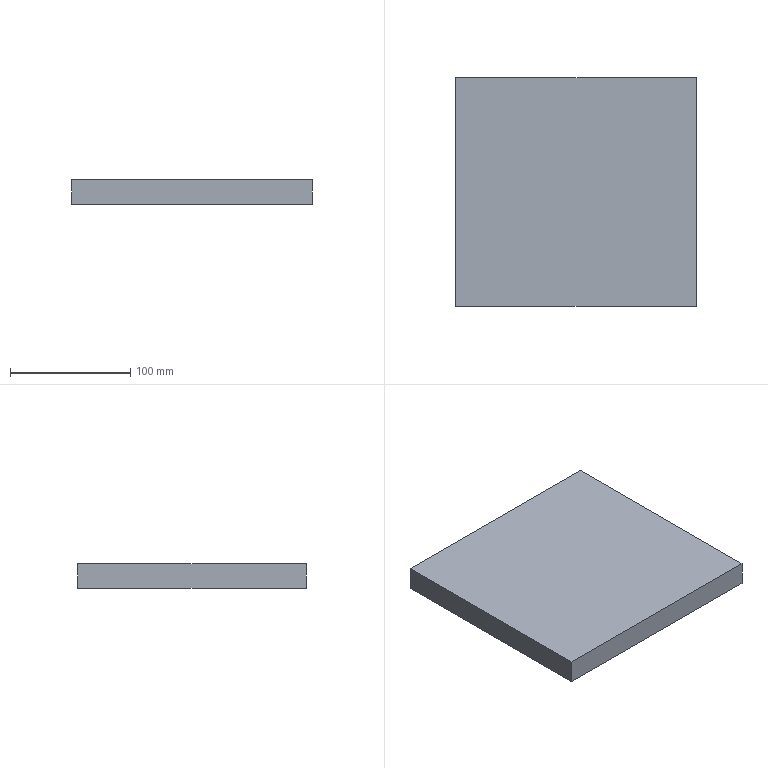Part | NX | features DATUM_CSYS 2, EXTRUDE 1, SKETCH 1 | 1 solid | 6 faces | box 200 x 190 x 20 mm | volume 760000 mm3 | plane 6
STEP:
#1=CARTESIAN_POINT('',(-100.,95.,0.));
#2=VERTEX_POINT('',#1);
#3=CARTESIAN_POINT('',(-100.,-95.,0.));
#4=VERTEX_POINT('',#3);
#5=CARTESIAN_POINT('',(-100.,95.,0.));
#6=DIRECTION('',(0.,-1.,0.));
#7=VECTOR('',#6,1000.);
#8=LINE('',#5,#7);
#9=EDGE_CURVE('',#2,#4,#8,.T.);
#10=ORIENTED_EDGE('',*,*,#9,.T.);
#11=CARTESIAN_POINT('',(-100.,-95.,20.));
#12=VERTEX_POINT('',#11);
#13=CARTESIAN_POINT('',(-100.,-95.,20.));
#14=DIRECTION('',(0.,0.,-1.));
#15=VECTOR('',#14,1000.);
#16=LINE('',#13,#15);
#17=EDGE_CURVE('',#12,#4,#16,.T.);
#18=ORIENTED_EDGE('',*,*,#17,.F.);
#19=CARTESIAN_POINT('',(-100.,95.,20.));
#20=VERTEX_POINT('',#19);
#21=CARTESIAN_POINT('',(-100.,95.,20.));
#22=DIRECTION('',(0.,-1.,0.));
#23=VECTOR('',#22,1000.);
#24=LINE('',#21,#23);
#25=EDGE_CURVE('',#20,#12,#24,.T.);
#26=ORIENTED_EDGE('',*,*,#25,.F.);
#27=CARTESIAN_POINT('',(-100.,95.,20.));
#28=DIRECTION('',(0.,0.,-1.));
#29=VECTOR('',#28,1000.);
#30=LINE('',#27,#29);
#31=EDGE_CURVE('',#20,#2,#30,.T.);
#32=ORIENTED_EDGE('',*,*,#31,.T.);
#33=EDGE_LOOP('',(#10,#18,#26,#32));
#34=FACE_BOUND('',#33,.T.);
#35=CARTESIAN_POINT('',(-100.,95.,20.));
#36=DIRECTION('',(1.,0.,0.));
#37=DIRECTION('',(0.,1.,0.));
#38=AXIS2_PLACEMENT_3D('',#35,#36,#37);
#39=PLANE('',#38);
#40=ADVANCED_FACE('',(#34),#39,.F.);
#41=CARTESIAN_POINT('',(100.,-95.,0.));
#42=VERTEX_POINT('',#41);
#43=CARTESIAN_POINT('',(-100.,-95.,0.));
#44=DIRECTION('',(1.,0.,0.));
#45=VECTOR('',#44,1000.);
#46=LINE('',#43,#45);
#47=EDGE_CURVE('',#4,#42,#46,.T.);
#48=ORIENTED_EDGE('',*,*,#47,.T.);
#49=CARTESIAN_POINT('',(100.,-95.,20.));
#50=VERTEX_POINT('',#49);
#51=CARTESIAN_POINT('',(100.,-95.,20.));
#52=DIRECTION('',(0.,0.,-1.));
#53=VECTOR('',#52,1000.);
#54=LINE('',#51,#53);
#55=EDGE_CURVE('',#50,#42,#54,.T.);
#56=ORIENTED_EDGE('',*,*,#55,.F.);
#57=CARTESIAN_POINT('',(-100.,-95.,20.));
#58=DIRECTION('',(1.,0.,0.));
#59=VECTOR('',#58,1000.);
#60=LINE('',#57,#59);
#61=EDGE_CURVE('',#12,#50,#60,.T.);
#62=ORIENTED_EDGE('',*,*,#61,.F.);
#63=ORIENTED_EDGE('',*,*,#17,.T.);
#64=EDGE_LOOP('',(#48,#56,#62,#63));
#65=FACE_BOUND('',#64,.T.);
#66=CARTESIAN_POINT('',(-100.,-95.,20.));
#67=DIRECTION('',(0.,1.,0.));
#68=DIRECTION('',(0.,0.,1.));
#69=AXIS2_PLACEMENT_3D('',#66,#67,#68);
#70=PLANE('',#69);
#71=ADVANCED_FACE('',(#65),#70,.F.);
#72=CARTESIAN_POINT('',(100.,95.,0.));
#73=VERTEX_POINT('',#72);
#74=CARTESIAN_POINT('',(100.,-95.,0.));
#75=DIRECTION('',(0.,1.,0.));
#76=VECTOR('',#75,1000.);
#77=LINE('',#74,#76);
#78=EDGE_CURVE('',#42,#73,#77,.T.);
#79=ORIENTED_EDGE('',*,*,#78,.T.);
#80=CARTESIAN_POINT('',(100.,95.,20.));
#81=VERTEX_POINT('',#80);
#82=CARTESIAN_POINT('',(100.,95.,20.));
#83=DIRECTION('',(0.,0.,-1.));
#84=VECTOR('',#83,1000.);
#85=LINE('',#82,#84);
#86=EDGE_CURVE('',#81,#73,#85,.T.);
#87=ORIENTED_EDGE('',*,*,#86,.F.);
#88=CARTESIAN_POINT('',(100.,-95.,20.));
#89=DIRECTION('',(0.,1.,0.));
#90=VECTOR('',#89,1000.);
#91=LINE('',#88,#90);
#92=EDGE_CURVE('',#50,#81,#91,.T.);
#93=ORIENTED_EDGE('',*,*,#92,.F.);
#94=ORIENTED_EDGE('',*,*,#55,.T.);
#95=EDGE_LOOP('',(#79,#87,#93,#94));
#96=FACE_BOUND('',#95,.T.);
#97=CARTESIAN_POINT('',(100.,-95.,20.));
#98=DIRECTION('',(-1.,0.,0.));
#99=DIRECTION('',(0.,-1.,0.));
#100=AXIS2_PLACEMENT_3D('',#97,#98,#99);
#101=PLANE('',#100);
#102=ADVANCED_FACE('',(#96),#101,.F.);
#103=CARTESIAN_POINT('',(100.,95.,0.));
#104=DIRECTION('',(-1.,0.,0.));
#105=VECTOR('',#104,1000.);
#106=LINE('',#103,#105);
#107=EDGE_CURVE('',#73,#2,#106,.T.);
#108=ORIENTED_EDGE('',*,*,#107,.T.);
#109=ORIENTED_EDGE('',*,*,#31,.F.);
#110=CARTESIAN_POINT('',(100.,95.,20.));
#111=DIRECTION('',(-1.,0.,0.));
#112=VECTOR('',#111,1000.);
#113=LINE('',#110,#112);
#114=EDGE_CURVE('',#81,#20,#113,.T.);
#115=ORIENTED_EDGE('',*,*,#114,.F.);
#116=ORIENTED_EDGE('',*,*,#86,.T.);
#117=EDGE_LOOP('',(#108,#109,#115,#116));
#118=FACE_BOUND('',#117,.T.);
#119=CARTESIAN_POINT('',(100.,95.,20.));
#120=DIRECTION('',(0.,-1.,0.));
#121=DIRECTION('',(0.,0.,-1.));
#122=AXIS2_PLACEMENT_3D('',#119,#120,#121);
#123=PLANE('',#122);
#124=ADVANCED_FACE('',(#118),#123,.F.);
#125=ORIENTED_EDGE('',*,*,#25,.T.);
#126=ORIENTED_EDGE('',*,*,#61,.T.);
#127=ORIENTED_EDGE('',*,*,#92,.T.);
#128=ORIENTED_EDGE('',*,*,#114,.T.);
#129=EDGE_LOOP('',(#125,#126,#127,#128));
#130=FACE_BOUND('',#129,.T.);
#131=CARTESIAN_POINT('',(0.,0.,20.));
#132=DIRECTION('',(0.,0.,1.));
#133=DIRECTION('',(1.,0.,0.));
#134=AXIS2_PLACEMENT_3D('',#131,#132,#133);
#135=PLANE('',#134);
#136=ADVANCED_FACE('',(#130),#135,.T.);
#137=ORIENTED_EDGE('',*,*,#9,.F.);
#138=ORIENTED_EDGE('',*,*,#107,.F.);
#139=ORIENTED_EDGE('',*,*,#78,.F.);
#140=ORIENTED_EDGE('',*,*,#47,.F.);
#141=EDGE_LOOP('',(#137,#138,#139,#140));
#142=FACE_BOUND('',#141,.T.);
#143=CARTESIAN_POINT('',(0.,0.,0.));
#144=DIRECTION('',(0.,0.,1.));
#145=DIRECTION('',(1.,0.,0.));
#146=AXIS2_PLACEMENT_3D('',#143,#144,#145);
#147=PLANE('',#146);
#148=ADVANCED_FACE('',(#142),#147,.F.);
#149=CLOSED_SHELL('',(#40,#71,#102,#124,#136,#148));
#150=MANIFOLD_SOLID_BREP('',#149);
#151=(LENGTH_UNIT()NAMED_UNIT(*)SI_UNIT(.MILLI.,.METRE.));
#152=UNCERTAINTY_MEASURE_WITH_UNIT(LENGTH_MEASURE(0.00001),#151,'','');
#153=(NAMED_UNIT(*)PLANE_ANGLE_UNIT()SI_UNIT($,.RADIAN.));
#154=(NAMED_UNIT(*)SI_UNIT($,.STERADIAN.)SOLID_ANGLE_UNIT());
#155=(GEOMETRIC_REPRESENTATION_CONTEXT(3)GLOBAL_UNCERTAINTY_ASSIGNED_CONTEXT((#152))GLOBAL_UNIT_ASSIGNED_CONTEXT((#151,#153,#154))REPRESENTATION_CONTEXT('',''));
#156=ADVANCED_BREP_SHAPE_REPRESENTATION('',(#150),#155);